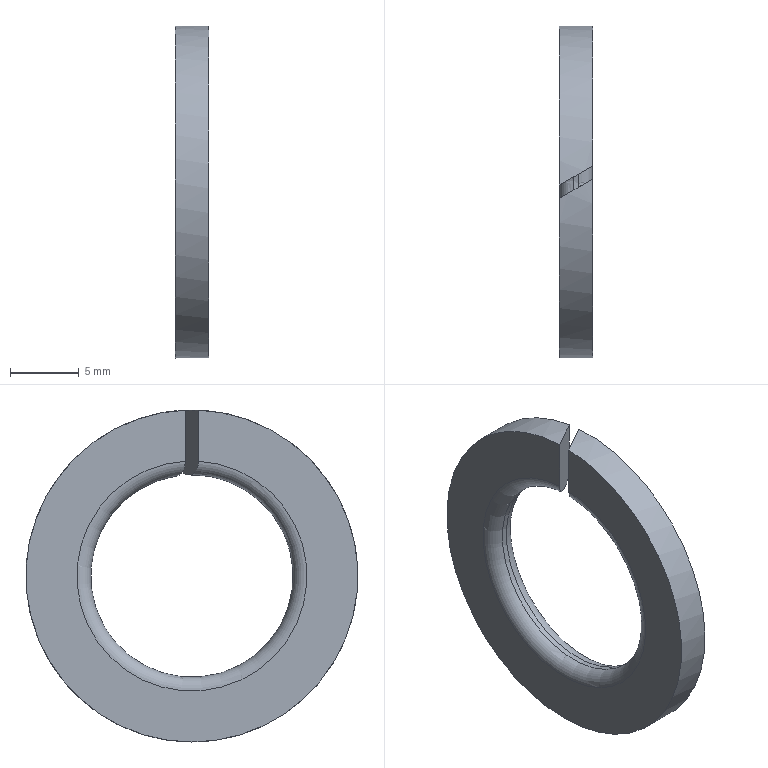Part | STEP file | DIN 128 - A14 | 1 solid | 8 faces | box 2.4 x 24.1 x 24.1 mm | volume 656.6 mm3 | plane 4 | cylinder 2 | torus 2 | commonest cylinder face diameters 14.7 x1 24.1 x1
STEP:
#1=CARTESIAN_POINT('',(0.,0.,0.));
#2=DIRECTION('',(0.,0.,1.));
#3=DIRECTION('',(1.,0.,0.));
#4=AXIS2_PLACEMENT_3D('',#1,#2,#3);
#5=CARTESIAN_POINT('',(2.4,1.866,8.139));
#6=VERTEX_POINT('',#5);
#7=CARTESIAN_POINT('',(1.4,1.288,7.236));
#8=VERTEX_POINT('',#7);
#9=CARTESIAN_POINT('',(2.4,1.866,8.139));
#10=CARTESIAN_POINT('',(2.4,1.866,8.019));
#11=CARTESIAN_POINT('',(2.374,1.85,7.878));
#12=CARTESIAN_POINT('',(2.285,1.799,7.66));
#13=CARTESIAN_POINT('',(2.207,1.754,7.547));
#14=CARTESIAN_POINT('',(2.039,1.657,7.387));
#15=CARTESIAN_POINT('',(1.917,1.587,7.316));
#16=CARTESIAN_POINT('',(1.684,1.452,7.238));
#17=CARTESIAN_POINT('',(1.529,1.363,7.223));
#18=CARTESIAN_POINT('',(1.4,1.288,7.236));
#19=B_SPLINE_CURVE_WITH_KNOTS('',3,(#9,#10,#11,#12,#13,#14,#15,#16,#17,#18),.UNSPECIFIED.,.F.,.F.,(4,2,2,2,4),(0.1663,0.2023,0.2385,0.2778,0.3227),.UNSPECIFIED.);
#20=CARTESIAN_POINT('',(0.,0.48,0.));
#21=DIRECTION('',(-0.5,0.866,0.));
#22=DIRECTION('',(0.,0.,1.));
#23=AXIS2_PLACEMENT_3D('',#20,#21,#22);
#24=PLANE('',#23);
#25=CARTESIAN_POINT('',(8.139,2.771));
#26=CARTESIAN_POINT('',(8.019,2.771));
#27=CARTESIAN_POINT('',(7.878,2.741));
#28=CARTESIAN_POINT('',(7.66,2.638));
#29=CARTESIAN_POINT('',(7.547,2.548));
#30=CARTESIAN_POINT('',(7.387,2.354));
#31=CARTESIAN_POINT('',(7.316,2.214));
#32=CARTESIAN_POINT('',(7.238,1.945));
#33=CARTESIAN_POINT('',(7.223,1.766));
#34=CARTESIAN_POINT('',(7.236,1.617));
#35=B_SPLINE_CURVE_WITH_KNOTS('',3,(#25,#26,#27,#28,#29,#30,#31,#32,#33,#34),.UNSPECIFIED.,.F.,.F.,(4,2,2,2,4),(0.1663,0.2023,0.2385,0.2778,0.3227),.UNSPECIFIED.);
#36=(GEOMETRIC_REPRESENTATION_CONTEXT(2)PARAMETRIC_REPRESENTATION_CONTEXT()REPRESENTATION_CONTEXT('',''));
#37=DEFINITIONAL_REPRESENTATION('',(#35),#36);
#38=PCURVE('',#24,#37);
#39=CARTESIAN_POINT('',(1.4,0.,0.));
#40=DIRECTION('',(-1.,0.,0.));
#41=DIRECTION('',(0.,0.,1.));
#42=AXIS2_PLACEMENT_3D('',#39,#40,#41);
#43=TOROIDAL_SURFACE('',#42,8.35,1.);
#44=CARTESIAN_POINT('',(0.2253,4.712));
#45=CARTESIAN_POINT('',(0.226,4.689));
#46=CARTESIAN_POINT('',(0.2272,4.641));
#47=CARTESIAN_POINT('',(0.2286,4.566));
#48=CARTESIAN_POINT('',(0.2298,4.489));
#49=CARTESIAN_POINT('',(0.2305,4.412));
#50=CARTESIAN_POINT('',(0.2308,4.339));
#51=CARTESIAN_POINT('',(0.2306,4.267));
#52=CARTESIAN_POINT('',(0.2298,4.19));
#53=CARTESIAN_POINT('',(0.2287,4.113));
#54=CARTESIAN_POINT('',(0.2271,4.037));
#55=CARTESIAN_POINT('',(0.2251,3.965));
#56=CARTESIAN_POINT('',(0.2228,3.896));
#57=CARTESIAN_POINT('',(0.2199,3.823));
#58=CARTESIAN_POINT('',(0.2166,3.75));
#59=CARTESIAN_POINT('',(0.213,3.677));
#60=CARTESIAN_POINT('',(0.2091,3.607));
#61=CARTESIAN_POINT('',(0.2052,3.542));
#62=CARTESIAN_POINT('',(0.2009,3.475));
#63=CARTESIAN_POINT('',(0.1962,3.407));
#64=CARTESIAN_POINT('',(0.1913,3.338));
#65=CARTESIAN_POINT('',(0.1862,3.27));
#66=CARTESIAN_POINT('',(0.1811,3.204));
#67=CARTESIAN_POINT('',(0.1778,3.162));
#68=CARTESIAN_POINT('',(0.1762,3.142));
#69=B_SPLINE_CURVE_WITH_KNOTS('',3,(#44,#45,#46,#47,#48,#49,#50,#51,#52,#53,#54,#55,#56,#57,#58,#59,#60,#61,#62,#63,#64,#65,#66,#67,#68),.UNSPECIFIED.,.F.,.F.,(4,1,1,1,1,1,1,1,1,1,1,1,1,1,1,1,1,1,1,1,1,1,4),(0.1663,0.1734,0.1805,0.1876,0.1947,0.2018,0.2089,0.2161,0.2232,0.2303,0.2374,0.2445,0.2516,0.2587,0.2658,0.2729,0.28,0.2871,0.2942,0.3014,0.3085,0.3156,0.3227),.QUASI_UNIFORM_KNOTS.);
#70=(GEOMETRIC_REPRESENTATION_CONTEXT(2)PARAMETRIC_REPRESENTATION_CONTEXT()REPRESENTATION_CONTEXT('',''));
#71=DEFINITIONAL_REPRESENTATION('',(#69),#70);
#72=PCURVE('',#43,#71);
#73=SURFACE_CURVE('',#19,(#38,#72),.PCURVE_S1.);
#74=EDGE_CURVE('',#6,#8,#73,.T.);
#75=ORIENTED_EDGE('',*,*,#74,.F.);
#76=CARTESIAN_POINT('',(2.4,1.866,11.905));
#77=VERTEX_POINT('',#76);
#78=CARTESIAN_POINT('',(2.4,1.866,0.));
#79=DIRECTION('',(0.,0.,-1.));
#80=VECTOR('',#79,1.);
#81=LINE('',#78,#80);
#82=CARTESIAN_POINT('',(0.,2.771));
#83=DIRECTION('',(-1.,0.));
#84=VECTOR('',#83,1.);
#85=LINE('',#82,#84);
#86=(GEOMETRIC_REPRESENTATION_CONTEXT(2)PARAMETRIC_REPRESENTATION_CONTEXT()REPRESENTATION_CONTEXT('',''));
#87=DEFINITIONAL_REPRESENTATION('',(#85),#86);
#88=PCURVE('',#24,#87);
#89=CARTESIAN_POINT('',(2.4,0.,0.));
#90=DIRECTION('',(-1.,0.,0.));
#91=DIRECTION('',(0.,0.,1.));
#92=AXIS2_PLACEMENT_3D('',#89,#90,#91);
#93=PLANE('',#92);
#94=CARTESIAN_POINT('',(0.,1.866));
#95=DIRECTION('',(-1.,0.));
#96=VECTOR('',#95,1.);
#97=LINE('',#94,#96);
#98=(GEOMETRIC_REPRESENTATION_CONTEXT(2)PARAMETRIC_REPRESENTATION_CONTEXT()REPRESENTATION_CONTEXT('',''));
#99=DEFINITIONAL_REPRESENTATION('',(#97),#98);
#100=PCURVE('',#93,#99);
#101=SURFACE_CURVE('',#81,(#88,#100),.PCURVE_S1.);
#102=EDGE_CURVE('',#77,#6,#101,.T.);
#103=ORIENTED_EDGE('',*,*,#102,.F.);
#104=CARTESIAN_POINT('',(0.,0.48,12.04));
#105=VERTEX_POINT('',#104);
#106=CARTESIAN_POINT('',(-0.8314,0.,0.));
#107=DIRECTION('',(-0.5,0.866,0.));
#108=DIRECTION('',(-0.866,-0.5,0.));
#109=AXIS2_PLACEMENT_3D('',#106,#107,#108);
#110=ELLIPSE('',#109,24.1,12.05);
#111=CARTESIAN_POINT('',(0.,-0.96));
#112=DIRECTION('',(0.,-1.));
#113=AXIS2_PLACEMENT_2D('',#111,#112);
#114=ELLIPSE('',#113,24.1,12.05);
#115=(GEOMETRIC_REPRESENTATION_CONTEXT(2)PARAMETRIC_REPRESENTATION_CONTEXT()REPRESENTATION_CONTEXT('',''));
#116=DEFINITIONAL_REPRESENTATION('',(#114),#115);
#117=PCURVE('',#24,#116);
#118=CARTESIAN_POINT('',(0.,0.,0.));
#119=DIRECTION('',(1.,0.,0.));
#120=DIRECTION('',(0.,-1.,0.));
#121=AXIS2_PLACEMENT_3D('',#118,#119,#120);
#122=CYLINDRICAL_SURFACE('',#121,12.05);
#123=CARTESIAN_POINT('',(4.673,0.));
#124=CARTESIAN_POINT('',(4.557,2.4));
#125=B_SPLINE_CURVE_WITH_KNOTS('',1,(#123,#124),.UNSPECIFIED.,.F.,.F.,(2,2),(1.611,1.726),.PIECEWISE_BEZIER_KNOTS.);
#126=(GEOMETRIC_REPRESENTATION_CONTEXT(2)PARAMETRIC_REPRESENTATION_CONTEXT()REPRESENTATION_CONTEXT('',''));
#127=DEFINITIONAL_REPRESENTATION('',(#125),#126);
#128=PCURVE('',#122,#127);
#129=SURFACE_CURVE('',#110,(#117,#128),.PCURVE_S1.);
#130=EDGE_CURVE('',#105,#77,#129,.T.);
#131=ORIENTED_EDGE('',*,*,#130,.F.);
#132=CARTESIAN_POINT('',(0.,0.48,8.336));
#133=VERTEX_POINT('',#132);
#134=CARTESIAN_POINT('',(0.,0.48,0.));
#135=DIRECTION('',(0.,0.,1.));
#136=VECTOR('',#135,1.);
#137=LINE('',#134,#136);
#138=CARTESIAN_POINT('',(0.,0.));
#139=DIRECTION('',(1.,0.));
#140=VECTOR('',#139,1.);
#141=LINE('',#138,#140);
#142=(GEOMETRIC_REPRESENTATION_CONTEXT(2)PARAMETRIC_REPRESENTATION_CONTEXT()REPRESENTATION_CONTEXT('',''));
#143=DEFINITIONAL_REPRESENTATION('',(#141),#142);
#144=PCURVE('',#24,#143);
#145=CARTESIAN_POINT('',(0.,0.,0.));
#146=DIRECTION('',(-1.,0.,0.));
#147=DIRECTION('',(0.,0.,1.));
#148=AXIS2_PLACEMENT_3D('',#145,#146,#147);
#149=PLANE('',#148);
#150=CARTESIAN_POINT('',(0.,0.48));
#151=DIRECTION('',(1.,0.));
#152=VECTOR('',#151,1.);
#153=LINE('',#150,#152);
#154=(GEOMETRIC_REPRESENTATION_CONTEXT(2)PARAMETRIC_REPRESENTATION_CONTEXT()REPRESENTATION_CONTEXT('',''));
#155=DEFINITIONAL_REPRESENTATION('',(#153),#154);
#156=PCURVE('',#149,#155);
#157=SURFACE_CURVE('',#137,(#144,#156),.PCURVE_S1.);
#158=EDGE_CURVE('',#133,#105,#157,.T.);
#159=ORIENTED_EDGE('',*,*,#158,.F.);
#160=CARTESIAN_POINT('',(1.,1.057,7.274));
#161=VERTEX_POINT('',#160);
#162=CARTESIAN_POINT('',(1.,1.057,7.274));
#163=CARTESIAN_POINT('',(0.8692,0.9818,7.285));
#164=CARTESIAN_POINT('',(0.7165,0.8937,7.328));
#165=CARTESIAN_POINT('',(0.4832,0.759,7.447));
#166=CARTESIAN_POINT('',(0.3589,0.6872,7.541));
#167=CARTESIAN_POINT('',(0.1897,0.5895,7.73));
#168=CARTESIAN_POINT('',(0.1114,0.5443,7.856));
#169=CARTESIAN_POINT('',(0.026,0.495,8.082));
#170=CARTESIAN_POINT('',(0.,0.48,8.219));
#171=CARTESIAN_POINT('',(0.,0.48,8.336));
#172=B_SPLINE_CURVE_WITH_KNOTS('',3,(#162,#163,#164,#165,#166,#167,#168,#169,#170,#171),.UNSPECIFIED.,.F.,.F.,(4,2,2,2,4),(0.3218,0.3672,0.4101,0.4488,0.484),.UNSPECIFIED.);
#173=CARTESIAN_POINT('',(7.274,1.155));
#174=CARTESIAN_POINT('',(7.285,1.004));
#175=CARTESIAN_POINT('',(7.328,0.8273));
#176=CARTESIAN_POINT('',(7.447,0.5579));
#177=CARTESIAN_POINT('',(7.541,0.4144));
#178=CARTESIAN_POINT('',(7.73,0.219));
#179=CARTESIAN_POINT('',(7.856,0.1286));
#180=CARTESIAN_POINT('',(8.082,0.03002));
#181=CARTESIAN_POINT('',(8.219,0.));
#182=CARTESIAN_POINT('',(8.336,0.));
#183=B_SPLINE_CURVE_WITH_KNOTS('',3,(#173,#174,#175,#176,#177,#178,#179,#180,#181,#182),.UNSPECIFIED.,.F.,.F.,(4,2,2,2,4),(0.3218,0.3672,0.4101,0.4488,0.484),.UNSPECIFIED.);
#184=(GEOMETRIC_REPRESENTATION_CONTEXT(2)PARAMETRIC_REPRESENTATION_CONTEXT()REPRESENTATION_CONTEXT('',''));
#185=DEFINITIONAL_REPRESENTATION('',(#183),#184);
#186=PCURVE('',#24,#185);
#187=CARTESIAN_POINT('',(1.,0.,0.));
#188=DIRECTION('',(1.,0.,0.));
#189=DIRECTION('',(0.,0.,-1.));
#190=AXIS2_PLACEMENT_3D('',#187,#188,#189);
#191=TOROIDAL_SURFACE('',#190,8.35,1.);
#192=CARTESIAN_POINT('',(9.28,3.142));
#193=CARTESIAN_POINT('',(9.282,3.163));
#194=CARTESIAN_POINT('',(9.286,3.206));
#195=CARTESIAN_POINT('',(9.291,3.274));
#196=CARTESIAN_POINT('',(9.297,3.344));
#197=CARTESIAN_POINT('',(9.302,3.413));
#198=CARTESIAN_POINT('',(9.308,3.481));
#199=CARTESIAN_POINT('',(9.313,3.547));
#200=CARTESIAN_POINT('',(9.318,3.611));
#201=CARTESIAN_POINT('',(9.323,3.68));
#202=CARTESIAN_POINT('',(9.328,3.751));
#203=CARTESIAN_POINT('',(9.333,3.823));
#204=CARTESIAN_POINT('',(9.338,3.894));
#205=CARTESIAN_POINT('',(9.342,3.961));
#206=CARTESIAN_POINT('',(9.346,4.03));
#207=CARTESIAN_POINT('',(9.35,4.104));
#208=CARTESIAN_POINT('',(9.353,4.18));
#209=CARTESIAN_POINT('',(9.357,4.256));
#210=CARTESIAN_POINT('',(9.359,4.329));
#211=CARTESIAN_POINT('',(9.362,4.401));
#212=CARTESIAN_POINT('',(9.364,4.479));
#213=CARTESIAN_POINT('',(9.365,4.558));
#214=CARTESIAN_POINT('',(9.367,4.637));
#215=CARTESIAN_POINT('',(9.367,4.688));
#216=CARTESIAN_POINT('',(9.367,4.712));
#217=B_SPLINE_CURVE_WITH_KNOTS('',3,(#192,#193,#194,#195,#196,#197,#198,#199,#200,#201,#202,#203,#204,#205,#206,#207,#208,#209,#210,#211,#212,#213,#214,#215,#216),.UNSPECIFIED.,.F.,.F.,(4,1,1,1,1,1,1,1,1,1,1,1,1,1,1,1,1,1,1,1,1,1,4),(0.3218,0.3292,0.3365,0.3439,0.3513,0.3587,0.366,0.3734,0.3808,0.3881,0.3955,0.4029,0.4103,0.4176,0.425,0.4324,0.4398,0.4471,0.4545,0.4619,0.4692,0.4766,0.484),.QUASI_UNIFORM_KNOTS.);
#218=(GEOMETRIC_REPRESENTATION_CONTEXT(2)PARAMETRIC_REPRESENTATION_CONTEXT()REPRESENTATION_CONTEXT('',''));
#219=DEFINITIONAL_REPRESENTATION('',(#217),#218);
#220=PCURVE('',#191,#219);
#221=SURFACE_CURVE('',#172,(#186,#220),.PCURVE_S1.);
#222=EDGE_CURVE('',#161,#133,#221,.T.);
#223=ORIENTED_EDGE('',*,*,#222,.F.);
#224=CARTESIAN_POINT('',(-0.8314,0.,0.));
#225=DIRECTION('',(0.5,-0.866,0.));
#226=DIRECTION('',(-0.866,-0.5,0.));
#227=AXIS2_PLACEMENT_3D('',#224,#225,#226);
#228=ELLIPSE('',#227,14.7,7.35);
#229=CARTESIAN_POINT('',(0.,-15.66));
#230=CARTESIAN_POINT('',(-12.731,-15.66));
#231=CARTESIAN_POINT('',(-6.365,6.39));
#232=CARTESIAN_POINT('',(0.,28.44));
#233=CARTESIAN_POINT('',(6.365,6.39));
#234=CARTESIAN_POINT('',(12.731,-15.66));
#235=CARTESIAN_POINT('',(0.,-15.66));
#236=(BOUNDED_CURVE()B_SPLINE_CURVE(2,(#229,#230,#231,#232,#233,#234,#235),.UNSPECIFIED.,.T.,.F.)B_SPLINE_CURVE_WITH_KNOTS((1,2,2,2,2,1),(-2.094,0.,2.094,4.189,6.283,8.378),.UNSPECIFIED.)CURVE()GEOMETRIC_REPRESENTATION_ITEM()RATIONAL_B_SPLINE_CURVE((1.,0.5,1.,0.5,1.,0.5,1.))REPRESENTATION_ITEM(''));
#237=(GEOMETRIC_REPRESENTATION_CONTEXT(2)PARAMETRIC_REPRESENTATION_CONTEXT()REPRESENTATION_CONTEXT('',''));
#238=DEFINITIONAL_REPRESENTATION('',(#236),#237);
#239=PCURVE('',#24,#238);
#240=CARTESIAN_POINT('',(0.,0.,0.));
#241=DIRECTION('',(1.,0.,0.));
#242=DIRECTION('',(0.,-1.,0.));
#243=AXIS2_PLACEMENT_3D('',#240,#241,#242);
#244=CYLINDRICAL_SURFACE('',#243,7.35);
#245=CARTESIAN_POINT('',(4.536,1.4));
#246=CARTESIAN_POINT('',(4.568,1.));
#247=B_SPLINE_CURVE_WITH_KNOTS('',1,(#245,#246),.UNSPECIFIED.,.F.,.F.,(2,2),(4.536,4.568),.PIECEWISE_BEZIER_KNOTS.);
#248=(GEOMETRIC_REPRESENTATION_CONTEXT(2)PARAMETRIC_REPRESENTATION_CONTEXT()REPRESENTATION_CONTEXT('',''));
#249=DEFINITIONAL_REPRESENTATION('',(#247),#248);
#250=PCURVE('',#244,#249);
#251=SURFACE_CURVE('',#228,(#239,#250),.PCURVE_S1.);
#252=EDGE_CURVE('',#8,#161,#251,.T.);
#253=ORIENTED_EDGE('',*,*,#252,.F.);
#254=EDGE_LOOP('',(#75,#103,#131,#159,#223,#253));
#255=FACE_BOUND('',#254,.T.);
#256=ADVANCED_FACE('',(#255),#24,.F.);
#257=CARTESIAN_POINT('',(1.4,0.3283,7.343));
#258=VERTEX_POINT('',#257);
#259=CARTESIAN_POINT('',(2.4,0.9056,8.301));
#260=VERTEX_POINT('',#259);
#261=CARTESIAN_POINT('',(1.4,0.3283,7.343));
#262=CARTESIAN_POINT('',(1.53,0.4034,7.339));
#263=CARTESIAN_POINT('',(1.685,0.4926,7.366));
#264=CARTESIAN_POINT('',(1.918,0.6274,7.46));
#265=CARTESIAN_POINT('',(2.041,0.6983,7.539));
#266=CARTESIAN_POINT('',(2.209,0.7954,7.71));
#267=CARTESIAN_POINT('',(2.287,0.8403,7.827));
#268=CARTESIAN_POINT('',(2.374,0.8906,8.046));
#269=CARTESIAN_POINT('',(2.4,0.9056,8.183));
#270=CARTESIAN_POINT('',(2.4,0.9056,8.301));
#271=B_SPLINE_CURVE_WITH_KNOTS('',3,(#261,#262,#263,#264,#265,#266,#267,#268,#269,#270),.UNSPECIFIED.,.F.,.F.,(4,2,2,2,4),(0.3195,0.3646,0.4052,0.4421,0.4774),.UNSPECIFIED.);
#272=CARTESIAN_POINT('',(2.4,0.9056,0.));
#273=DIRECTION('',(0.5,-0.866,0.));
#274=DIRECTION('',(0.,0.,-1.));
#275=AXIS2_PLACEMENT_3D('',#272,#273,#274);
#276=PLANE('',#275);
#277=CARTESIAN_POINT('',(-7.343,-1.155));
#278=CARTESIAN_POINT('',(-7.339,-1.004));
#279=CARTESIAN_POINT('',(-7.366,-0.8261));
#280=CARTESIAN_POINT('',(-7.46,-0.5565));
#281=CARTESIAN_POINT('',(-7.539,-0.4147));
#282=CARTESIAN_POINT('',(-7.71,-0.2205));
#283=CARTESIAN_POINT('',(-7.827,-0.1306));
#284=CARTESIAN_POINT('',(-8.046,-0.03015));
#285=CARTESIAN_POINT('',(-8.183,0.));
#286=CARTESIAN_POINT('',(-8.301,0.));
#287=B_SPLINE_CURVE_WITH_KNOTS('',3,(#277,#278,#279,#280,#281,#282,#283,#284,#285,#286),.UNSPECIFIED.,.F.,.F.,(4,2,2,2,4),(0.3195,0.3646,0.4052,0.4421,0.4774),.UNSPECIFIED.);
#288=(GEOMETRIC_REPRESENTATION_CONTEXT(2)PARAMETRIC_REPRESENTATION_CONTEXT()REPRESENTATION_CONTEXT('',''));
#289=DEFINITIONAL_REPRESENTATION('',(#287),#288);
#290=PCURVE('',#276,#289);
#291=CARTESIAN_POINT('',(6.328,3.142));
#292=CARTESIAN_POINT('',(6.329,3.162));
#293=CARTESIAN_POINT('',(6.333,3.205));
#294=CARTESIAN_POINT('',(6.338,3.272));
#295=CARTESIAN_POINT('',(6.343,3.34));
#296=CARTESIAN_POINT('',(6.348,3.409));
#297=CARTESIAN_POINT('',(6.353,3.477));
#298=CARTESIAN_POINT('',(6.358,3.543));
#299=CARTESIAN_POINT('',(6.362,3.608));
#300=CARTESIAN_POINT('',(6.366,3.677));
#301=CARTESIAN_POINT('',(6.371,3.749));
#302=CARTESIAN_POINT('',(6.375,3.821));
#303=CARTESIAN_POINT('',(6.378,3.893));
#304=CARTESIAN_POINT('',(6.381,3.962));
#305=CARTESIAN_POINT('',(6.384,4.032));
#306=CARTESIAN_POINT('',(6.387,4.108));
#307=CARTESIAN_POINT('',(6.389,4.184));
#308=CARTESIAN_POINT('',(6.391,4.261));
#309=CARTESIAN_POINT('',(6.392,4.334));
#310=CARTESIAN_POINT('',(6.393,4.406));
#311=CARTESIAN_POINT('',(6.393,4.483));
#312=CARTESIAN_POINT('',(6.393,4.562));
#313=CARTESIAN_POINT('',(6.393,4.639));
#314=CARTESIAN_POINT('',(6.392,4.689));
#315=CARTESIAN_POINT('',(6.392,4.712));
#316=B_SPLINE_CURVE_WITH_KNOTS('',3,(#291,#292,#293,#294,#295,#296,#297,#298,#299,#300,#301,#302,#303,#304,#305,#306,#307,#308,#309,#310,#311,#312,#313,#314,#315),.UNSPECIFIED.,.F.,.F.,(4,1,1,1,1,1,1,1,1,1,1,1,1,1,1,1,1,1,1,1,1,1,4),(0.3195,0.3267,0.3339,0.3411,0.3482,0.3554,0.3626,0.3698,0.3769,0.3841,0.3913,0.3985,0.4056,0.4128,0.42,0.4272,0.4343,0.4415,0.4487,0.4559,0.463,0.4702,0.4774),.QUASI_UNIFORM_KNOTS.);
#317=(GEOMETRIC_REPRESENTATION_CONTEXT(2)PARAMETRIC_REPRESENTATION_CONTEXT()REPRESENTATION_CONTEXT('',''));
#318=DEFINITIONAL_REPRESENTATION('',(#316),#317);
#319=PCURVE('',#43,#318);
#320=SURFACE_CURVE('',#271,(#290,#319),.PCURVE_S1.);
#321=EDGE_CURVE('',#258,#260,#320,.T.);
#322=ORIENTED_EDGE('',*,*,#321,.F.);
#323=CARTESIAN_POINT('',(1.,0.09735,7.349));
#324=VERTEX_POINT('',#323);
#325=CARTESIAN_POINT('',(0.8314,0.,0.));
#326=DIRECTION('',(-0.5,0.866,0.));
#327=DIRECTION('',(-0.866,-0.5,0.));
#328=AXIS2_PLACEMENT_3D('',#325,#326,#327);
#329=ELLIPSE('',#328,14.7,7.35);
#330=CARTESIAN_POINT('',(0.,-16.511));
#331=CARTESIAN_POINT('',(-12.731,-16.511));
#332=CARTESIAN_POINT('',(-6.365,5.539));
#333=CARTESIAN_POINT('',(0.,27.589));
#334=CARTESIAN_POINT('',(6.365,5.539));
#335=CARTESIAN_POINT('',(12.731,-16.511));
#336=CARTESIAN_POINT('',(0.,-16.511));
#337=(BOUNDED_CURVE()B_SPLINE_CURVE(2,(#330,#331,#332,#333,#334,#335,#336),.UNSPECIFIED.,.T.,.F.)B_SPLINE_CURVE_WITH_KNOTS((1,2,2,2,2,1),(-2.094,0.,2.094,4.189,6.283,8.378),.UNSPECIFIED.)CURVE()GEOMETRIC_REPRESENTATION_ITEM()RATIONAL_B_SPLINE_CURVE((1.,0.5,1.,0.5,1.,0.5,1.))REPRESENTATION_ITEM(''));
#338=(GEOMETRIC_REPRESENTATION_CONTEXT(2)PARAMETRIC_REPRESENTATION_CONTEXT()REPRESENTATION_CONTEXT('',''));
#339=DEFINITIONAL_REPRESENTATION('',(#337),#338);
#340=PCURVE('',#276,#339);
#341=CARTESIAN_POINT('',(-1.584,1.));
#342=CARTESIAN_POINT('',(-1.615,1.4));
#343=B_SPLINE_CURVE_WITH_KNOTS('',1,(#341,#342),.UNSPECIFIED.,.F.,.F.,(2,2),(1.584,1.615),.PIECEWISE_BEZIER_KNOTS.);
#344=(GEOMETRIC_REPRESENTATION_CONTEXT(2)PARAMETRIC_REPRESENTATION_CONTEXT()REPRESENTATION_CONTEXT('',''));
#345=DEFINITIONAL_REPRESENTATION('',(#343),#344);
#346=PCURVE('',#244,#345);
#347=SURFACE_CURVE('',#329,(#340,#346),.PCURVE_S1.);
#348=EDGE_CURVE('',#324,#258,#347,.T.);
#349=ORIENTED_EDGE('',*,*,#348,.F.);
#350=CARTESIAN_POINT('',(0.,-0.48,8.336));
#351=VERTEX_POINT('',#350);
#352=CARTESIAN_POINT('',(0.,-0.48,8.336));
#353=CARTESIAN_POINT('',(0.,-0.48,8.219));
#354=CARTESIAN_POINT('',(0.02604,-0.465,8.082));
#355=CARTESIAN_POINT('',(0.1124,-0.4151,7.862));
#356=CARTESIAN_POINT('',(0.1904,-0.3701,7.743));
#357=CARTESIAN_POINT('',(0.3588,-0.2729,7.567));
#358=CARTESIAN_POINT('',(0.482,-0.2017,7.483));
#359=CARTESIAN_POINT('',(0.7156,-0.06687,7.382));
#360=CARTESIAN_POINT('',(0.8696,0.02207,7.35));
#361=CARTESIAN_POINT('',(1.,0.09735,7.349));
#362=B_SPLINE_CURVE_WITH_KNOTS('',3,(#352,#353,#354,#355,#356,#357,#358,#359,#360,#361),.UNSPECIFIED.,.F.,.F.,(4,2,2,2,4),(0.1607,0.1958,0.2331,0.2744,0.3196),.UNSPECIFIED.);
#363=CARTESIAN_POINT('',(-8.336,-2.771));
#364=CARTESIAN_POINT('',(-8.219,-2.771));
#365=CARTESIAN_POINT('',(-8.082,-2.741));
#366=CARTESIAN_POINT('',(-7.862,-2.641));
#367=CARTESIAN_POINT('',(-7.743,-2.551));
#368=CARTESIAN_POINT('',(-7.567,-2.357));
#369=CARTESIAN_POINT('',(-7.483,-2.215));
#370=CARTESIAN_POINT('',(-7.382,-1.945));
#371=CARTESIAN_POINT('',(-7.35,-1.767));
#372=CARTESIAN_POINT('',(-7.349,-1.617));
#373=B_SPLINE_CURVE_WITH_KNOTS('',3,(#363,#364,#365,#366,#367,#368,#369,#370,#371,#372),.UNSPECIFIED.,.F.,.F.,(4,2,2,2,4),(0.1607,0.1958,0.2331,0.2744,0.3196),.UNSPECIFIED.);
#374=(GEOMETRIC_REPRESENTATION_CONTEXT(2)PARAMETRIC_REPRESENTATION_CONTEXT()REPRESENTATION_CONTEXT('',''));
#375=DEFINITIONAL_REPRESENTATION('',(#373),#374);
#376=PCURVE('',#276,#375);
#377=CARTESIAN_POINT('',(3.199,4.712));
#378=CARTESIAN_POINT('',(3.199,4.688));
#379=CARTESIAN_POINT('',(3.199,4.639));
#380=CARTESIAN_POINT('',(3.199,4.56));
#381=CARTESIAN_POINT('',(3.199,4.482));
#382=CARTESIAN_POINT('',(3.198,4.404));
#383=CARTESIAN_POINT('',(3.197,4.332));
#384=CARTESIAN_POINT('',(3.195,4.259));
#385=CARTESIAN_POINT('',(3.193,4.182));
#386=CARTESIAN_POINT('',(3.19,4.106));
#387=CARTESIAN_POINT('',(3.187,4.031));
#388=CARTESIAN_POINT('',(3.184,3.961));
#389=CARTESIAN_POINT('',(3.181,3.893));
#390=CARTESIAN_POINT('',(3.177,3.821));
#391=CARTESIAN_POINT('',(3.172,3.749));
#392=CARTESIAN_POINT('',(3.168,3.678));
#393=CARTESIAN_POINT('',(3.163,3.608));
#394=CARTESIAN_POINT('',(3.159,3.544));
#395=CARTESIAN_POINT('',(3.154,3.478));
#396=CARTESIAN_POINT('',(3.149,3.41));
#397=CARTESIAN_POINT('',(3.144,3.341));
#398=CARTESIAN_POINT('',(3.139,3.272));
#399=CARTESIAN_POINT('',(3.133,3.205));
#400=CARTESIAN_POINT('',(3.13,3.162));
#401=CARTESIAN_POINT('',(3.128,3.142));
#402=B_SPLINE_CURVE_WITH_KNOTS('',3,(#377,#378,#379,#380,#381,#382,#383,#384,#385,#386,#387,#388,#389,#390,#391,#392,#393,#394,#395,#396,#397,#398,#399,#400,#401),.UNSPECIFIED.,.F.,.F.,(4,1,1,1,1,1,1,1,1,1,1,1,1,1,1,1,1,1,1,1,1,1,4),(0.1607,0.1679,0.1751,0.1823,0.1896,0.1968,0.204,0.2112,0.2185,0.2257,0.2329,0.2401,0.2473,0.2546,0.2618,0.269,0.2762,0.2835,0.2907,0.2979,0.3051,0.3123,0.3196),.QUASI_UNIFORM_KNOTS.);
#403=(GEOMETRIC_REPRESENTATION_CONTEXT(2)PARAMETRIC_REPRESENTATION_CONTEXT()REPRESENTATION_CONTEXT('',''));
#404=DEFINITIONAL_REPRESENTATION('',(#402),#403);
#405=PCURVE('',#191,#404);
#406=SURFACE_CURVE('',#362,(#376,#405),.PCURVE_S1.);
#407=EDGE_CURVE('',#351,#324,#406,.T.);
#408=ORIENTED_EDGE('',*,*,#407,.F.);
#409=CARTESIAN_POINT('',(0.,-0.48,12.04));
#410=VERTEX_POINT('',#409);
#411=CARTESIAN_POINT('',(0.,-0.48,0.));
#412=DIRECTION('',(0.,0.,-1.));
#413=VECTOR('',#412,1.);
#414=LINE('',#411,#413);
#415=CARTESIAN_POINT('',(0.,-2.771));
#416=DIRECTION('',(1.,0.));
#417=VECTOR('',#416,1.);
#418=LINE('',#415,#417);
#419=(GEOMETRIC_REPRESENTATION_CONTEXT(2)PARAMETRIC_REPRESENTATION_CONTEXT()REPRESENTATION_CONTEXT('',''));
#420=DEFINITIONAL_REPRESENTATION('',(#418),#419);
#421=PCURVE('',#276,#420);
#422=CARTESIAN_POINT('',(0.,-0.48));
#423=DIRECTION('',(-1.,0.));
#424=VECTOR('',#423,1.);
#425=LINE('',#422,#424);
#426=(GEOMETRIC_REPRESENTATION_CONTEXT(2)PARAMETRIC_REPRESENTATION_CONTEXT()REPRESENTATION_CONTEXT('',''));
#427=DEFINITIONAL_REPRESENTATION('',(#425),#426);
#428=PCURVE('',#149,#427);
#429=SURFACE_CURVE('',#414,(#421,#428),.PCURVE_S1.);
#430=EDGE_CURVE('',#410,#351,#429,.T.);
#431=ORIENTED_EDGE('',*,*,#430,.F.);
#432=CARTESIAN_POINT('',(2.4,0.9056,12.016));
#433=VERTEX_POINT('',#432);
#434=CARTESIAN_POINT('',(0.8314,0.,0.));
#435=DIRECTION('',(0.5,-0.866,0.));
#436=DIRECTION('',(-0.866,-0.5,0.));
#437=AXIS2_PLACEMENT_3D('',#434,#435,#436);
#438=ELLIPSE('',#437,24.1,12.05);
#439=CARTESIAN_POINT('',(0.,-1.811));
#440=DIRECTION('',(0.,-1.));
#441=AXIS2_PLACEMENT_2D('',#439,#440);
#442=ELLIPSE('',#441,24.1,12.05);
#443=(GEOMETRIC_REPRESENTATION_CONTEXT(2)PARAMETRIC_REPRESENTATION_CONTEXT()REPRESENTATION_CONTEXT('',''));
#444=DEFINITIONAL_REPRESENTATION('',(#442),#443);
#445=PCURVE('',#276,#444);
#446=CARTESIAN_POINT('',(-1.646,2.4));
#447=CARTESIAN_POINT('',(-1.531,0.));
#448=B_SPLINE_CURVE_WITH_KNOTS('',1,(#446,#447),.UNSPECIFIED.,.F.,.F.,(2,2),(4.637,4.752),.PIECEWISE_BEZIER_KNOTS.);
#449=(GEOMETRIC_REPRESENTATION_CONTEXT(2)PARAMETRIC_REPRESENTATION_CONTEXT()REPRESENTATION_CONTEXT('',''));
#450=DEFINITIONAL_REPRESENTATION('',(#448),#449);
#451=PCURVE('',#122,#450);
#452=SURFACE_CURVE('',#438,(#445,#451),.PCURVE_S1.);
#453=EDGE_CURVE('',#433,#410,#452,.T.);
#454=ORIENTED_EDGE('',*,*,#453,.F.);
#455=CARTESIAN_POINT('',(2.4,0.9056,0.));
#456=DIRECTION('',(0.,0.,1.));
#457=VECTOR('',#456,1.);
#458=LINE('',#455,#457);
#459=CARTESIAN_POINT('',(0.,0.));
#460=DIRECTION('',(-1.,0.));
#461=VECTOR('',#460,1.);
#462=LINE('',#459,#461);
#463=(GEOMETRIC_REPRESENTATION_CONTEXT(2)PARAMETRIC_REPRESENTATION_CONTEXT()REPRESENTATION_CONTEXT('',''));
#464=DEFINITIONAL_REPRESENTATION('',(#462),#463);
#465=PCURVE('',#276,#464);
#466=CARTESIAN_POINT('',(0.,0.9056));
#467=DIRECTION('',(1.,0.));
#468=VECTOR('',#467,1.);
#469=LINE('',#466,#468);
#470=(GEOMETRIC_REPRESENTATION_CONTEXT(2)PARAMETRIC_REPRESENTATION_CONTEXT()REPRESENTATION_CONTEXT('',''));
#471=DEFINITIONAL_REPRESENTATION('',(#469),#470);
#472=PCURVE('',#93,#471);
#473=SURFACE_CURVE('',#458,(#465,#472),.PCURVE_S1.);
#474=EDGE_CURVE('',#260,#433,#473,.T.);
#475=ORIENTED_EDGE('',*,*,#474,.F.);
#476=EDGE_LOOP('',(#322,#349,#408,#431,#454,#475));
#477=FACE_BOUND('',#476,.T.);
#478=ADVANCED_FACE('',(#477),#276,.F.);
#479=CARTESIAN_POINT('',(1.4,0.,0.));
#480=DIRECTION('',(-1.,0.,0.));
#481=DIRECTION('',(0.,-1.,0.));
#482=AXIS2_PLACEMENT_3D('',#479,#480,#481);
#483=CIRCLE('',#482,7.35);
#484=CARTESIAN_POINT('',(6.283,1.4));
#485=DIRECTION('',(-1.,0.));
#486=VECTOR('',#485,1.);
#487=LINE('',#484,#486);
#488=(GEOMETRIC_REPRESENTATION_CONTEXT(2)PARAMETRIC_REPRESENTATION_CONTEXT()REPRESENTATION_CONTEXT('',''));
#489=DEFINITIONAL_REPRESENTATION('',(#487),#488);
#490=PCURVE('',#244,#489);
#491=CARTESIAN_POINT('',(-1.571,3.142));
#492=DIRECTION('',(1.,0.));
#493=VECTOR('',#492,1.);
#494=LINE('',#491,#493);
#495=(GEOMETRIC_REPRESENTATION_CONTEXT(2)PARAMETRIC_REPRESENTATION_CONTEXT()REPRESENTATION_CONTEXT('',''));
#496=DEFINITIONAL_REPRESENTATION('',(#494),#495);
#497=PCURVE('',#43,#496);
#498=SURFACE_CURVE('',#483,(#490,#497),.PCURVE_S1.);
#499=EDGE_CURVE('',#8,#258,#498,.T.);
#500=ORIENTED_EDGE('',*,*,#499,.T.);
#501=ORIENTED_EDGE('',*,*,#348,.F.);
#502=CARTESIAN_POINT('',(1.,0.,0.));
#503=DIRECTION('',(1.,0.,0.));
#504=DIRECTION('',(0.,-1.,0.));
#505=AXIS2_PLACEMENT_3D('',#502,#503,#504);
#506=CIRCLE('',#505,7.35);
#507=CARTESIAN_POINT('',(-6.283,1.));
#508=DIRECTION('',(1.,0.));
#509=VECTOR('',#508,1.);
#510=LINE('',#507,#509);
#511=(GEOMETRIC_REPRESENTATION_CONTEXT(2)PARAMETRIC_REPRESENTATION_CONTEXT()REPRESENTATION_CONTEXT('',''));
#512=DEFINITIONAL_REPRESENTATION('',(#510),#511);
#513=PCURVE('',#244,#512);
#514=CARTESIAN_POINT('',(-1.571,3.142));
#515=DIRECTION('',(1.,0.));
#516=VECTOR('',#515,1.);
#517=LINE('',#514,#516);
#518=(GEOMETRIC_REPRESENTATION_CONTEXT(2)PARAMETRIC_REPRESENTATION_CONTEXT()REPRESENTATION_CONTEXT('',''));
#519=DEFINITIONAL_REPRESENTATION('',(#517),#518);
#520=PCURVE('',#191,#519);
#521=SURFACE_CURVE('',#506,(#513,#520),.PCURVE_S1.);
#522=EDGE_CURVE('',#324,#161,#521,.T.);
#523=ORIENTED_EDGE('',*,*,#522,.T.);
#524=ORIENTED_EDGE('',*,*,#252,.F.);
#525=EDGE_LOOP('',(#500,#501,#523,#524));
#526=FACE_BOUND('',#525,.F.);
#527=ADVANCED_FACE('',(#526),#244,.F.);
#528=ORIENTED_EDGE('',*,*,#222,.T.);
#529=CARTESIAN_POINT('',(0.,0.,0.));
#530=DIRECTION('',(-1.,0.,0.));
#531=DIRECTION('',(0.,-1.,0.));
#532=AXIS2_PLACEMENT_3D('',#529,#530,#531);
#533=CIRCLE('',#532,8.35);
#534=CARTESIAN_POINT('',(10.996,4.712));
#535=DIRECTION('',(-1.,0.));
#536=VECTOR('',#535,1.);
#537=LINE('',#534,#536);
#538=(GEOMETRIC_REPRESENTATION_CONTEXT(2)PARAMETRIC_REPRESENTATION_CONTEXT()REPRESENTATION_CONTEXT('',''));
#539=DEFINITIONAL_REPRESENTATION('',(#537),#538);
#540=PCURVE('',#191,#539);
#541=CARTESIAN_POINT('',(0.,0.));
#542=DIRECTION('',(0.,-1.));
#543=AXIS2_PLACEMENT_2D('',#541,#542);
#544=CIRCLE('',#543,8.35);
#545=(GEOMETRIC_REPRESENTATION_CONTEXT(2)PARAMETRIC_REPRESENTATION_CONTEXT()REPRESENTATION_CONTEXT('',''));
#546=DEFINITIONAL_REPRESENTATION('',(#544),#545);
#547=PCURVE('',#149,#546);
#548=SURFACE_CURVE('',#533,(#540,#547),.PCURVE_S1.);
#549=EDGE_CURVE('',#133,#351,#548,.T.);
#550=ORIENTED_EDGE('',*,*,#549,.T.);
#551=ORIENTED_EDGE('',*,*,#407,.T.);
#552=ORIENTED_EDGE('',*,*,#522,.T.);
#553=EDGE_LOOP('',(#528,#550,#551,#552));
#554=FACE_BOUND('',#553,.T.);
#555=ADVANCED_FACE('',(#554),#191,.T.);
#556=ORIENTED_EDGE('',*,*,#158,.T.);
#557=CARTESIAN_POINT('',(0.,0.,0.));
#558=DIRECTION('',(-1.,0.,0.));
#559=DIRECTION('',(0.,-1.,0.));
#560=AXIS2_PLACEMENT_3D('',#557,#558,#559);
#561=CIRCLE('',#560,12.05);
#562=CARTESIAN_POINT('',(0.,0.));
#563=DIRECTION('',(0.,-1.));
#564=AXIS2_PLACEMENT_2D('',#562,#563);
#565=CIRCLE('',#564,12.05);
#566=(GEOMETRIC_REPRESENTATION_CONTEXT(2)PARAMETRIC_REPRESENTATION_CONTEXT()REPRESENTATION_CONTEXT('',''));
#567=DEFINITIONAL_REPRESENTATION('',(#565),#566);
#568=PCURVE('',#149,#567);
#569=CARTESIAN_POINT('',(6.283,0.));
#570=DIRECTION('',(-1.,0.));
#571=VECTOR('',#570,1.);
#572=LINE('',#569,#571);
#573=(GEOMETRIC_REPRESENTATION_CONTEXT(2)PARAMETRIC_REPRESENTATION_CONTEXT()REPRESENTATION_CONTEXT('',''));
#574=DEFINITIONAL_REPRESENTATION('',(#572),#573);
#575=PCURVE('',#122,#574);
#576=SURFACE_CURVE('',#561,(#568,#575),.PCURVE_S1.);
#577=EDGE_CURVE('',#105,#410,#576,.T.);
#578=ORIENTED_EDGE('',*,*,#577,.T.);
#579=ORIENTED_EDGE('',*,*,#430,.T.);
#580=ORIENTED_EDGE('',*,*,#549,.F.);
#581=EDGE_LOOP('',(#556,#578,#579,#580));
#582=FACE_BOUND('',#581,.T.);
#583=ADVANCED_FACE('',(#582),#149,.T.);
#584=ORIENTED_EDGE('',*,*,#74,.T.);
#585=ORIENTED_EDGE('',*,*,#499,.T.);
#586=ORIENTED_EDGE('',*,*,#321,.T.);
#587=CARTESIAN_POINT('',(2.4,0.,0.));
#588=DIRECTION('',(1.,0.,0.));
#589=DIRECTION('',(0.,-1.,0.));
#590=AXIS2_PLACEMENT_3D('',#587,#588,#589);
#591=CIRCLE('',#590,8.35);
#592=CARTESIAN_POINT('',(10.996,4.712));
#593=DIRECTION('',(-1.,0.));
#594=VECTOR('',#593,1.);
#595=LINE('',#592,#594);
#596=(GEOMETRIC_REPRESENTATION_CONTEXT(2)PARAMETRIC_REPRESENTATION_CONTEXT()REPRESENTATION_CONTEXT('',''));
#597=DEFINITIONAL_REPRESENTATION('',(#595),#596);
#598=PCURVE('',#43,#597);
#599=CARTESIAN_POINT('',(0.,-8.35));
#600=CARTESIAN_POINT('',(-14.463,-8.35));
#601=CARTESIAN_POINT('',(-7.231,4.175));
#602=CARTESIAN_POINT('',(0.,16.7));
#603=CARTESIAN_POINT('',(7.231,4.175));
#604=CARTESIAN_POINT('',(14.463,-8.35));
#605=CARTESIAN_POINT('',(0.,-8.35));
#606=(BOUNDED_CURVE()B_SPLINE_CURVE(2,(#599,#600,#601,#602,#603,#604,#605),.UNSPECIFIED.,.T.,.F.)B_SPLINE_CURVE_WITH_KNOTS((1,2,2,2,2,1),(-2.094,0.,2.094,4.189,6.283,8.378),.UNSPECIFIED.)CURVE()GEOMETRIC_REPRESENTATION_ITEM()RATIONAL_B_SPLINE_CURVE((1.,0.5,1.,0.5,1.,0.5,1.))REPRESENTATION_ITEM(''));
#607=(GEOMETRIC_REPRESENTATION_CONTEXT(2)PARAMETRIC_REPRESENTATION_CONTEXT()REPRESENTATION_CONTEXT('',''));
#608=DEFINITIONAL_REPRESENTATION('',(#606),#607);
#609=PCURVE('',#93,#608);
#610=SURFACE_CURVE('',#591,(#598,#609),.PCURVE_S1.);
#611=EDGE_CURVE('',#260,#6,#610,.T.);
#612=ORIENTED_EDGE('',*,*,#611,.T.);
#613=EDGE_LOOP('',(#584,#585,#586,#612));
#614=FACE_BOUND('',#613,.T.);
#615=ADVANCED_FACE('',(#614),#43,.T.);
#616=ORIENTED_EDGE('',*,*,#102,.T.);
#617=ORIENTED_EDGE('',*,*,#611,.F.);
#618=ORIENTED_EDGE('',*,*,#474,.T.);
#619=CARTESIAN_POINT('',(2.4,0.,0.));
#620=DIRECTION('',(-1.,0.,0.));
#621=DIRECTION('',(0.,-1.,0.));
#622=AXIS2_PLACEMENT_3D('',#619,#620,#621);
#623=CIRCLE('',#622,12.05);
#624=CARTESIAN_POINT('',(0.,0.));
#625=DIRECTION('',(0.,-1.));
#626=AXIS2_PLACEMENT_2D('',#624,#625);
#627=CIRCLE('',#626,12.05);
#628=(GEOMETRIC_REPRESENTATION_CONTEXT(2)PARAMETRIC_REPRESENTATION_CONTEXT()REPRESENTATION_CONTEXT('',''));
#629=DEFINITIONAL_REPRESENTATION('',(#627),#628);
#630=PCURVE('',#93,#629);
#631=CARTESIAN_POINT('',(6.283,2.4));
#632=DIRECTION('',(-1.,0.));
#633=VECTOR('',#632,1.);
#634=LINE('',#631,#633);
#635=(GEOMETRIC_REPRESENTATION_CONTEXT(2)PARAMETRIC_REPRESENTATION_CONTEXT()REPRESENTATION_CONTEXT('',''));
#636=DEFINITIONAL_REPRESENTATION('',(#634),#635);
#637=PCURVE('',#122,#636);
#638=SURFACE_CURVE('',#623,(#630,#637),.PCURVE_S1.);
#639=EDGE_CURVE('',#77,#433,#638,.T.);
#640=ORIENTED_EDGE('',*,*,#639,.F.);
#641=EDGE_LOOP('',(#616,#617,#618,#640));
#642=FACE_BOUND('',#641,.T.);
#643=ADVANCED_FACE('',(#642),#93,.F.);
#644=ORIENTED_EDGE('',*,*,#130,.T.);
#645=ORIENTED_EDGE('',*,*,#639,.T.);
#646=ORIENTED_EDGE('',*,*,#453,.T.);
#647=ORIENTED_EDGE('',*,*,#577,.F.);
#648=EDGE_LOOP('',(#644,#645,#646,#647));
#649=FACE_BOUND('',#648,.T.);
#650=ADVANCED_FACE('',(#649),#122,.T.);
#651=CLOSED_SHELL('',(#256,#478,#527,#555,#583,#615,#643,#650));
#652=MANIFOLD_SOLID_BREP('',#651);
#653=(LENGTH_UNIT()NAMED_UNIT(*)SI_UNIT(.MILLI.,.METRE.));
#654=UNCERTAINTY_MEASURE_WITH_UNIT(LENGTH_MEASURE(0.001),#653,'','');
#655=(NAMED_UNIT(*)PLANE_ANGLE_UNIT()SI_UNIT($,.RADIAN.));
#656=(NAMED_UNIT(*)SI_UNIT($,.STERADIAN.)SOLID_ANGLE_UNIT());
#657=(GEOMETRIC_REPRESENTATION_CONTEXT(3)GLOBAL_UNCERTAINTY_ASSIGNED_CONTEXT((#654))GLOBAL_UNIT_ASSIGNED_CONTEXT((#653,#655,#656))REPRESENTATION_CONTEXT('',''));
#658=ADVANCED_BREP_SHAPE_REPRESENTATION('',(#4,#652),#657);